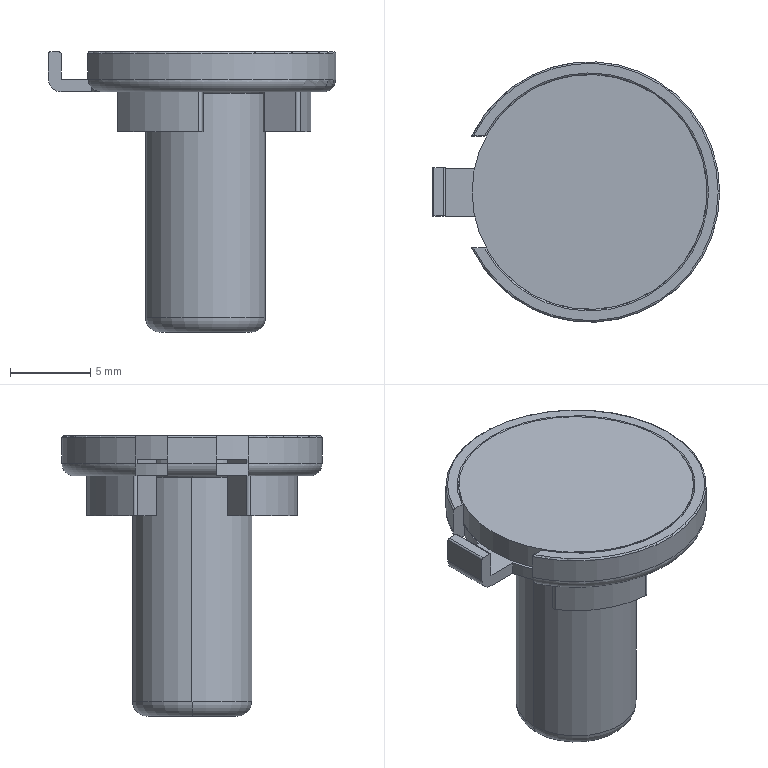CAM job | NX | 3-axis milling, drilling | part box 17.958 x 16.273 x 17.5 mm
Tools:
number,name,description,diameter,corner_radius,flute_length,length,flutes
4,D4,Milling Tool-5 Parameters,4.0,0.0,50.0,75.0,2
2,D2,Milling Tool-5 Parameters,2.0,0.0,50.0,75.0,2
7,D4A45,Milling Tool-5 Parameters,4.0,0.0,50.0,75.0,2
1,ZXZ,Milling Tool-5 Parameters,6.0,0.0,50.0,75.0,2
11,1.0ZT,Drilling Tool,1.0,0.0,35.0,50.0,2
5,D4R0.5,Milling Tool-5 Parameters,4.0,0.5,50.0,75.0,2
12,D1,Milling Tool-5 Parameters,1.0,0.0,50.0,75.0,2
Operations:
program,operation,operation_type,tool,method,geometry_group,spindle_rpm,surface_speed,feed_per_tooth,feed_cut,feed_plunge,cut_length_mm,path_length_mm,cut_time_min,machine_time_min
1,ZLEVEL_PROFILE_COPY,ZLevelMilling,D4,METHOD,A,6500.0,81.0,0.1385,1800.0,100.0,157.644,211.62,0.0876,0.093
1,ZLEVEL_PROFILE_COPY_COPY_1,ZLevelMilling,D4,METHOD,A,6500.0,81.0,0.0769,1000.0,100.0,7.358,31.758,0.0074,0.0098
1,ZLEVEL_PROFILE_COPY_COPY,ZLevelMilling,D4,METHOD,A,6500.0,40.0,0.1385,1800.0,100.0,2213.903,2280.604,1.23,1.237
1,ZLEVEL_PROFILE_COPY_COPY_COPY,ZLevelMilling,D4,METHOD,A,6500.0,40.0,0.0769,1000.0,100.0,68.913,94.913,0.0689,0.0715
1,ZLEVEL_PROFILE_COPY_1,ZLevelMilling,D2,METHOD,A,6500.0,40.0,0.0962,1250.0,100.0,378.284,681.212,0.3026,0.3329
1,ZLEVEL_PROFILE,ZLevelMilling,D2,METHOD,A,6500.0,40.0,0.0962,1250.0,100.0,807.366,896.449,0.6459,0.6548
1,ZLEVEL_PROFILE_COPY_1_1,ZLevelMilling,D1,METHOD,A,6500.0,20.0,0.0654,850.0,100.0,1256.585,1819.773,1.478,1.535
1,ZLEVEL_PROFILE_COPY_1_1_COPY,ZLevelMilling,D1,METHOD,A,6500.0,20.0,0.0654,850.0,100.0,270.461,440.555,0.3182,0.3352
1,PLANAR_MILL,PlanarMilling,D4A45,METHOD,A,7500.0,94.0,0.0833,1250.0,100.0,67.401,108.816,0.0539,0.0581
2,DRILLING,Operation,ZXZ,METHOD,B,5000.0,94.0,0.025,250.0,0.0,28.4,161.255,0.1136,0.1269
2,DRILLING_COPY,Operation,1.0ZT,METHOD,B,2000.0,6.0,0.025,100.0,0.0,44.803,194.062,0.448,0.463
2,ZLEVEL_PROFILE_1,ZLevelMilling,D4R0.5,METHOD,B,7500.0,94.0,0.1667,2500.0,1000.0,1331.686,1420.996,0.5339,0.5429
FIXTURE,ZLEVEL_PROFILE_COPY_COPY_2_COPY,ZLevelMilling,D4,METHOD,C,6500.0,81.0,0.1385,1800.0,100.0,811.953,874.953,0.4511,0.4574
FIXTURE,ZLEVEL_PROFILE_COPY_COPY_2,ZLevelMilling,D4,METHOD,C,6500.0,81.0,0.1385,1800.0,100.0,591.536,653.036,0.3286,0.3348
FIXTURE,ZLEVEL_PROFILE_COPY_COPY_2_COPY_1,ZLevelMilling,D2,METHOD,C,8000.0,50.0,0.0625,1000.0,100.0,335.173,917.483,0.3352,0.3934
FIXTURE,ZLEVEL_PROFILE_COPY_COPY_2_COPY_1_COPY,ZLevelMilling,D1,METHOD,C,8005.0,25.0,0.0531,850.0,100.0,1644.976,19348.942,1.935,3.706
FIXTURE,刀补,ZLevelMilling,D4,METHOD,C,6500.0,81.0,0.0769,1000.0,100.0,107.632,174.132,0.1076,0.1143
FIXTURE,刀补1,ZLevelMilling,D4,METHOD,C,6500.0,81.0,0.0769,1000.0,100.0,219.309,280.809,0.2193,0.2255
FIXTURE,刀补2,ZLevelMilling,D1,METHOD,C,6500.0,20.0,0.0654,850.0,100.0,513.034,787.573,0.6036,0.631